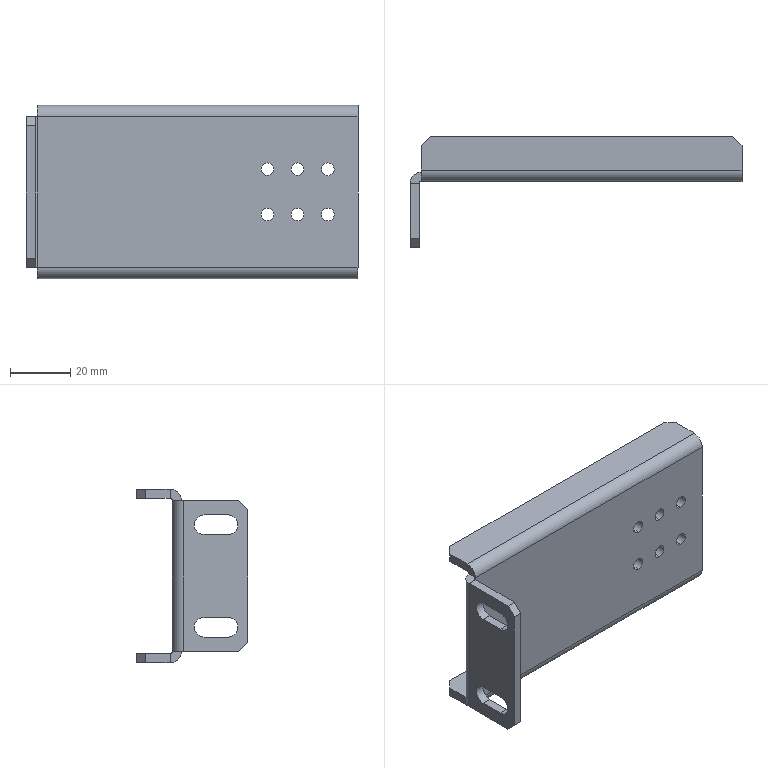Part | STEP file | 11-FG-SJ01411 | 1 solid | 56 faces | box 110 x 37 x 57.473 mm | volume 28236 mm3 | plane 34 | cylinder 22 | commonest cylinder face diameters 4.2 x12 6.5 x4 1.473 x3 7.473 x3